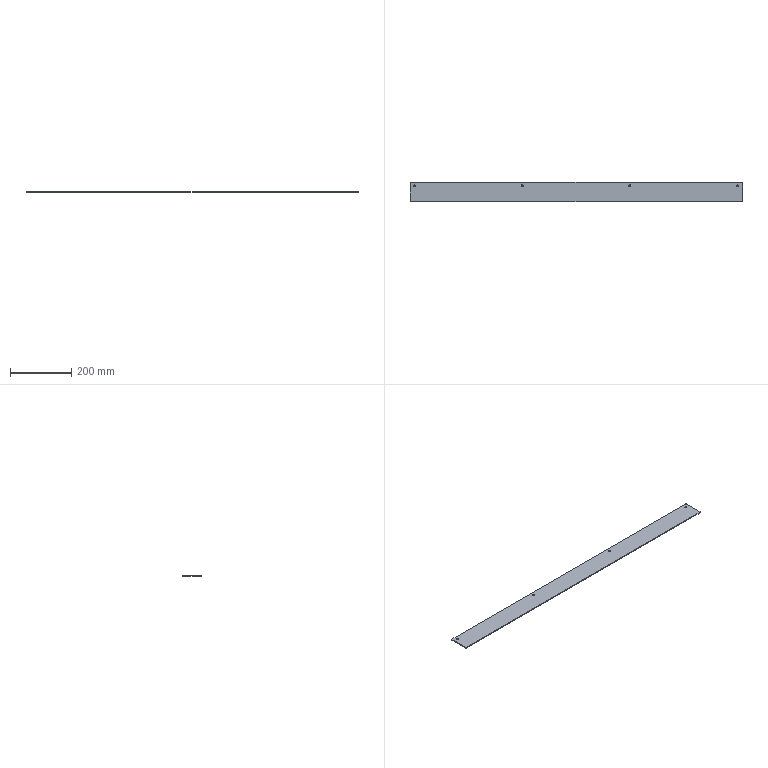Part | NX | features BREP 1 | 1 solid | 18 faces | box 1080 x 65 x 3 mm | volume 210250 mm3 | cylinder 12 | plane 6 | commonest cylinder face diameters 6 x8 4 x4
STEP:
#1=CARTESIAN_POINT('',(540.,-30.5,-3.));
#2=VERTEX_POINT('',#1);
#3=CARTESIAN_POINT('',(538.,-32.5,-3.));
#4=VERTEX_POINT('',#3);
#5=CARTESIAN_POINT('',(538.,-30.5,-3.));
#6=DIRECTION('',(0.,0.,-1.));
#7=DIRECTION('',(-1.,0.,0.));
#8=AXIS2_PLACEMENT_3D('',#5,#6,#7);
#9=CIRCLE('',#8,2.);
#10=EDGE_CURVE('',#2,#4,#9,.T.);
#11=ORIENTED_EDGE('',*,*,#10,.F.);
#12=CARTESIAN_POINT('',(540.,-30.5,0.));
#13=VERTEX_POINT('',#12);
#14=CARTESIAN_POINT('',(540.,-30.5,-3.));
#15=DIRECTION('',(0.,0.,-1.));
#16=VECTOR('',#15,1000.);
#17=LINE('',#14,#16);
#18=EDGE_CURVE('',#13,#2,#17,.T.);
#19=ORIENTED_EDGE('',*,*,#18,.F.);
#20=CARTESIAN_POINT('',(538.,-32.5,0.));
#21=VERTEX_POINT('',#20);
#22=CARTESIAN_POINT('',(538.,-30.5,0.));
#23=DIRECTION('',(0.,0.,1.));
#24=DIRECTION('',(-1.,0.,0.));
#25=AXIS2_PLACEMENT_3D('',#22,#23,#24);
#26=CIRCLE('',#25,2.);
#27=EDGE_CURVE('',#21,#13,#26,.T.);
#28=ORIENTED_EDGE('',*,*,#27,.F.);
#29=CARTESIAN_POINT('',(538.,-32.5,-3.));
#30=DIRECTION('',(0.,0.,1.));
#31=VECTOR('',#30,1000.);
#32=LINE('',#29,#31);
#33=EDGE_CURVE('',#4,#21,#32,.T.);
#34=ORIENTED_EDGE('',*,*,#33,.F.);
#35=EDGE_LOOP('',(#11,#19,#28,#34));
#36=FACE_BOUND('',#35,.T.);
#37=CARTESIAN_POINT('',(538.,-30.5,-3.));
#38=DIRECTION('',(0.,0.,1.));
#39=DIRECTION('',(1.,0.,0.));
#40=AXIS2_PLACEMENT_3D('',#37,#38,#39);
#41=CYLINDRICAL_SURFACE('',#40,2.);
#42=ADVANCED_FACE('',(#36),#41,.T.);
#43=CARTESIAN_POINT('',(538.,32.5,-3.));
#44=VERTEX_POINT('',#43);
#45=CARTESIAN_POINT('',(540.,30.5,-3.));
#46=VERTEX_POINT('',#45);
#47=CARTESIAN_POINT('',(538.,30.5,-3.));
#48=DIRECTION('',(0.,0.,-1.));
#49=DIRECTION('',(-1.,0.,0.));
#50=AXIS2_PLACEMENT_3D('',#47,#48,#49);
#51=CIRCLE('',#50,2.);
#52=EDGE_CURVE('',#44,#46,#51,.T.);
#53=ORIENTED_EDGE('',*,*,#52,.F.);
#54=CARTESIAN_POINT('',(538.,32.5,0.));
#55=VERTEX_POINT('',#54);
#56=CARTESIAN_POINT('',(538.,32.5,-3.));
#57=DIRECTION('',(0.,0.,-1.));
#58=VECTOR('',#57,1000.);
#59=LINE('',#56,#58);
#60=EDGE_CURVE('',#55,#44,#59,.T.);
#61=ORIENTED_EDGE('',*,*,#60,.F.);
#62=CARTESIAN_POINT('',(540.,30.5,0.));
#63=VERTEX_POINT('',#62);
#64=CARTESIAN_POINT('',(538.,30.5,0.));
#65=DIRECTION('',(0.,0.,1.));
#66=DIRECTION('',(-1.,0.,0.));
#67=AXIS2_PLACEMENT_3D('',#64,#65,#66);
#68=CIRCLE('',#67,2.);
#69=EDGE_CURVE('',#63,#55,#68,.T.);
#70=ORIENTED_EDGE('',*,*,#69,.F.);
#71=CARTESIAN_POINT('',(540.,30.5,-3.));
#72=DIRECTION('',(0.,0.,1.));
#73=VECTOR('',#72,1000.);
#74=LINE('',#71,#73);
#75=EDGE_CURVE('',#46,#63,#74,.T.);
#76=ORIENTED_EDGE('',*,*,#75,.F.);
#77=EDGE_LOOP('',(#53,#61,#70,#76));
#78=FACE_BOUND('',#77,.T.);
#79=CARTESIAN_POINT('',(538.,30.5,-3.));
#80=DIRECTION('',(0.,0.,1.));
#81=DIRECTION('',(1.,0.,0.));
#82=AXIS2_PLACEMENT_3D('',#79,#80,#81);
#83=CYLINDRICAL_SURFACE('',#82,2.);
#84=ADVANCED_FACE('',(#78),#83,.T.);
#85=CARTESIAN_POINT('',(-538.,-32.5,-3.));
#86=VERTEX_POINT('',#85);
#87=CARTESIAN_POINT('',(-540.,-30.5,-3.));
#88=VERTEX_POINT('',#87);
#89=CARTESIAN_POINT('',(-538.,-30.5,-3.));
#90=DIRECTION('',(0.,0.,-1.));
#91=DIRECTION('',(-1.,0.,0.));
#92=AXIS2_PLACEMENT_3D('',#89,#90,#91);
#93=CIRCLE('',#92,2.);
#94=EDGE_CURVE('',#86,#88,#93,.T.);
#95=ORIENTED_EDGE('',*,*,#94,.F.);
#96=CARTESIAN_POINT('',(-538.,-32.5,0.));
#97=VERTEX_POINT('',#96);
#98=CARTESIAN_POINT('',(-538.,-32.5,-3.));
#99=DIRECTION('',(0.,0.,-1.));
#100=VECTOR('',#99,1000.);
#101=LINE('',#98,#100);
#102=EDGE_CURVE('',#97,#86,#101,.T.);
#103=ORIENTED_EDGE('',*,*,#102,.F.);
#104=CARTESIAN_POINT('',(-540.,-30.5,0.));
#105=VERTEX_POINT('',#104);
#106=CARTESIAN_POINT('',(-538.,-30.5,0.));
#107=DIRECTION('',(0.,0.,1.));
#108=DIRECTION('',(-1.,0.,0.));
#109=AXIS2_PLACEMENT_3D('',#106,#107,#108);
#110=CIRCLE('',#109,2.);
#111=EDGE_CURVE('',#105,#97,#110,.T.);
#112=ORIENTED_EDGE('',*,*,#111,.F.);
#113=CARTESIAN_POINT('',(-540.,-30.5,-3.));
#114=DIRECTION('',(0.,0.,1.));
#115=VECTOR('',#114,1000.);
#116=LINE('',#113,#115);
#117=EDGE_CURVE('',#88,#105,#116,.T.);
#118=ORIENTED_EDGE('',*,*,#117,.F.);
#119=EDGE_LOOP('',(#95,#103,#112,#118));
#120=FACE_BOUND('',#119,.T.);
#121=CARTESIAN_POINT('',(-538.,-30.5,-3.));
#122=DIRECTION('',(0.,0.,1.));
#123=DIRECTION('',(1.,0.,0.));
#124=AXIS2_PLACEMENT_3D('',#121,#122,#123);
#125=CYLINDRICAL_SURFACE('',#124,2.);
#126=ADVANCED_FACE('',(#120),#125,.T.);
#127=CARTESIAN_POINT('',(-540.,30.5,-3.));
#128=VERTEX_POINT('',#127);
#129=CARTESIAN_POINT('',(-538.,32.5,-3.));
#130=VERTEX_POINT('',#129);
#131=CARTESIAN_POINT('',(-538.,30.5,-3.));
#132=DIRECTION('',(0.,0.,-1.));
#133=DIRECTION('',(-1.,0.,0.));
#134=AXIS2_PLACEMENT_3D('',#131,#132,#133);
#135=CIRCLE('',#134,2.);
#136=EDGE_CURVE('',#128,#130,#135,.T.);
#137=ORIENTED_EDGE('',*,*,#136,.F.);
#138=CARTESIAN_POINT('',(-540.,30.5,0.));
#139=VERTEX_POINT('',#138);
#140=CARTESIAN_POINT('',(-540.,30.5,-3.));
#141=DIRECTION('',(0.,0.,-1.));
#142=VECTOR('',#141,1000.);
#143=LINE('',#140,#142);
#144=EDGE_CURVE('',#139,#128,#143,.T.);
#145=ORIENTED_EDGE('',*,*,#144,.F.);
#146=CARTESIAN_POINT('',(-538.,32.5,0.));
#147=VERTEX_POINT('',#146);
#148=CARTESIAN_POINT('',(-538.,30.5,0.));
#149=DIRECTION('',(0.,0.,1.));
#150=DIRECTION('',(-1.,0.,0.));
#151=AXIS2_PLACEMENT_3D('',#148,#149,#150);
#152=CIRCLE('',#151,2.);
#153=EDGE_CURVE('',#147,#139,#152,.T.);
#154=ORIENTED_EDGE('',*,*,#153,.F.);
#155=CARTESIAN_POINT('',(-538.,32.5,-3.));
#156=DIRECTION('',(0.,0.,1.));
#157=VECTOR('',#156,1000.);
#158=LINE('',#155,#157);
#159=EDGE_CURVE('',#130,#147,#158,.T.);
#160=ORIENTED_EDGE('',*,*,#159,.F.);
#161=EDGE_LOOP('',(#137,#145,#154,#160));
#162=FACE_BOUND('',#161,.T.);
#163=CARTESIAN_POINT('',(-538.,30.5,-3.));
#164=DIRECTION('',(0.,0.,1.));
#165=DIRECTION('',(1.,0.,0.));
#166=AXIS2_PLACEMENT_3D('',#163,#164,#165);
#167=CYLINDRICAL_SURFACE('',#166,2.);
#168=ADVANCED_FACE('',(#162),#167,.T.);
#169=CARTESIAN_POINT('',(528.,20.,0.));
#170=VERTEX_POINT('',#169);
#171=CARTESIAN_POINT('',(528.,20.,-3.));
#172=VERTEX_POINT('',#171);
#173=CARTESIAN_POINT('',(528.,20.,-3.));
#174=DIRECTION('',(0.,0.,-1.));
#175=VECTOR('',#174,1000.);
#176=LINE('',#173,#175);
#177=EDGE_CURVE('',#170,#172,#176,.T.);
#178=ORIENTED_EDGE('',*,*,#177,.F.);
#179=CARTESIAN_POINT('',(522.,20.,0.));
#180=VERTEX_POINT('',#179);
#181=CARTESIAN_POINT('',(525.,20.,0.));
#182=DIRECTION('',(0.,0.,-1.));
#183=DIRECTION('',(-1.,0.,0.));
#184=AXIS2_PLACEMENT_3D('',#181,#182,#183);
#185=CIRCLE('',#184,3.);
#186=EDGE_CURVE('',#180,#170,#185,.T.);
#187=ORIENTED_EDGE('',*,*,#186,.F.);
#188=CARTESIAN_POINT('',(522.,20.,-3.));
#189=VERTEX_POINT('',#188);
#190=CARTESIAN_POINT('',(522.,20.,-3.));
#191=DIRECTION('',(0.,0.,-1.));
#192=VECTOR('',#191,1000.);
#193=LINE('',#190,#192);
#194=EDGE_CURVE('',#180,#189,#193,.T.);
#195=ORIENTED_EDGE('',*,*,#194,.T.);
#196=CARTESIAN_POINT('',(525.,20.,-3.));
#197=DIRECTION('',(0.,0.,-1.));
#198=DIRECTION('',(-1.,0.,0.));
#199=AXIS2_PLACEMENT_3D('',#196,#197,#198);
#200=CIRCLE('',#199,3.);
#201=EDGE_CURVE('',#189,#172,#200,.T.);
#202=ORIENTED_EDGE('',*,*,#201,.T.);
#203=EDGE_LOOP('',(#178,#187,#195,#202));
#204=FACE_BOUND('',#203,.T.);
#205=CARTESIAN_POINT('',(525.,20.,-3.));
#206=DIRECTION('',(0.,0.,-1.));
#207=DIRECTION('',(-1.,0.,0.));
#208=AXIS2_PLACEMENT_3D('',#205,#206,#207);
#209=CYLINDRICAL_SURFACE('',#208,3.);
#210=ADVANCED_FACE('',(#204),#209,.F.);
#211=CARTESIAN_POINT('',(178.,20.,0.));
#212=VERTEX_POINT('',#211);
#213=CARTESIAN_POINT('',(178.,20.,-3.));
#214=VERTEX_POINT('',#213);
#215=CARTESIAN_POINT('',(178.,20.,-3.));
#216=DIRECTION('',(0.,0.,-1.));
#217=VECTOR('',#216,1000.);
#218=LINE('',#215,#217);
#219=EDGE_CURVE('',#212,#214,#218,.T.);
#220=ORIENTED_EDGE('',*,*,#219,.F.);
#221=CARTESIAN_POINT('',(172.,20.,0.));
#222=VERTEX_POINT('',#221);
#223=CARTESIAN_POINT('',(175.,20.,0.));
#224=DIRECTION('',(0.,0.,-1.));
#225=DIRECTION('',(-1.,0.,0.));
#226=AXIS2_PLACEMENT_3D('',#223,#224,#225);
#227=CIRCLE('',#226,3.);
#228=EDGE_CURVE('',#222,#212,#227,.T.);
#229=ORIENTED_EDGE('',*,*,#228,.F.);
#230=CARTESIAN_POINT('',(172.,20.,-3.));
#231=VERTEX_POINT('',#230);
#232=CARTESIAN_POINT('',(172.,20.,-3.));
#233=DIRECTION('',(0.,0.,-1.));
#234=VECTOR('',#233,1000.);
#235=LINE('',#232,#234);
#236=EDGE_CURVE('',#222,#231,#235,.T.);
#237=ORIENTED_EDGE('',*,*,#236,.T.);
#238=CARTESIAN_POINT('',(175.,20.,-3.));
#239=DIRECTION('',(0.,0.,-1.));
#240=DIRECTION('',(-1.,0.,0.));
#241=AXIS2_PLACEMENT_3D('',#238,#239,#240);
#242=CIRCLE('',#241,3.);
#243=EDGE_CURVE('',#231,#214,#242,.T.);
#244=ORIENTED_EDGE('',*,*,#243,.T.);
#245=EDGE_LOOP('',(#220,#229,#237,#244));
#246=FACE_BOUND('',#245,.T.);
#247=CARTESIAN_POINT('',(175.,20.,-3.));
#248=DIRECTION('',(0.,0.,-1.));
#249=DIRECTION('',(-1.,0.,0.));
#250=AXIS2_PLACEMENT_3D('',#247,#248,#249);
#251=CYLINDRICAL_SURFACE('',#250,3.);
#252=ADVANCED_FACE('',(#246),#251,.F.);
#253=CARTESIAN_POINT('',(-172.,20.,0.));
#254=VERTEX_POINT('',#253);
#255=CARTESIAN_POINT('',(-172.,20.,-3.));
#256=VERTEX_POINT('',#255);
#257=CARTESIAN_POINT('',(-172.,20.,-3.));
#258=DIRECTION('',(0.,0.,-1.));
#259=VECTOR('',#258,1000.);
#260=LINE('',#257,#259);
#261=EDGE_CURVE('',#254,#256,#260,.T.);
#262=ORIENTED_EDGE('',*,*,#261,.F.);
#263=CARTESIAN_POINT('',(-178.,20.,0.));
#264=VERTEX_POINT('',#263);
#265=CARTESIAN_POINT('',(-175.,20.,0.));
#266=DIRECTION('',(0.,0.,-1.));
#267=DIRECTION('',(-1.,0.,0.));
#268=AXIS2_PLACEMENT_3D('',#265,#266,#267);
#269=CIRCLE('',#268,3.);
#270=EDGE_CURVE('',#264,#254,#269,.T.);
#271=ORIENTED_EDGE('',*,*,#270,.F.);
#272=CARTESIAN_POINT('',(-178.,20.,-3.));
#273=VERTEX_POINT('',#272);
#274=CARTESIAN_POINT('',(-178.,20.,-3.));
#275=DIRECTION('',(0.,0.,-1.));
#276=VECTOR('',#275,1000.);
#277=LINE('',#274,#276);
#278=EDGE_CURVE('',#264,#273,#277,.T.);
#279=ORIENTED_EDGE('',*,*,#278,.T.);
#280=CARTESIAN_POINT('',(-175.,20.,-3.));
#281=DIRECTION('',(0.,0.,-1.));
#282=DIRECTION('',(-1.,0.,0.));
#283=AXIS2_PLACEMENT_3D('',#280,#281,#282);
#284=CIRCLE('',#283,3.);
#285=EDGE_CURVE('',#273,#256,#284,.T.);
#286=ORIENTED_EDGE('',*,*,#285,.T.);
#287=EDGE_LOOP('',(#262,#271,#279,#286));
#288=FACE_BOUND('',#287,.T.);
#289=CARTESIAN_POINT('',(-175.,20.,-3.));
#290=DIRECTION('',(0.,0.,-1.));
#291=DIRECTION('',(-1.,0.,0.));
#292=AXIS2_PLACEMENT_3D('',#289,#290,#291);
#293=CYLINDRICAL_SURFACE('',#292,3.);
#294=ADVANCED_FACE('',(#288),#293,.F.);
#295=CARTESIAN_POINT('',(-522.,20.,0.));
#296=VERTEX_POINT('',#295);
#297=CARTESIAN_POINT('',(-522.,20.,-3.));
#298=VERTEX_POINT('',#297);
#299=CARTESIAN_POINT('',(-522.,20.,-3.));
#300=DIRECTION('',(0.,0.,-1.));
#301=VECTOR('',#300,1000.);
#302=LINE('',#299,#301);
#303=EDGE_CURVE('',#296,#298,#302,.T.);
#304=ORIENTED_EDGE('',*,*,#303,.F.);
#305=CARTESIAN_POINT('',(-528.,20.,0.));
#306=VERTEX_POINT('',#305);
#307=CARTESIAN_POINT('',(-525.,20.,0.));
#308=DIRECTION('',(0.,0.,-1.));
#309=DIRECTION('',(-1.,0.,0.));
#310=AXIS2_PLACEMENT_3D('',#307,#308,#309);
#311=CIRCLE('',#310,3.);
#312=EDGE_CURVE('',#306,#296,#311,.T.);
#313=ORIENTED_EDGE('',*,*,#312,.F.);
#314=CARTESIAN_POINT('',(-528.,20.,-3.));
#315=VERTEX_POINT('',#314);
#316=CARTESIAN_POINT('',(-528.,20.,-3.));
#317=DIRECTION('',(0.,0.,-1.));
#318=VECTOR('',#317,1000.);
#319=LINE('',#316,#318);
#320=EDGE_CURVE('',#306,#315,#319,.T.);
#321=ORIENTED_EDGE('',*,*,#320,.T.);
#322=CARTESIAN_POINT('',(-525.,20.,-3.));
#323=DIRECTION('',(0.,0.,-1.));
#324=DIRECTION('',(-1.,0.,0.));
#325=AXIS2_PLACEMENT_3D('',#322,#323,#324);
#326=CIRCLE('',#325,3.);
#327=EDGE_CURVE('',#315,#298,#326,.T.);
#328=ORIENTED_EDGE('',*,*,#327,.T.);
#329=EDGE_LOOP('',(#304,#313,#321,#328));
#330=FACE_BOUND('',#329,.T.);
#331=CARTESIAN_POINT('',(-525.,20.,-3.));
#332=DIRECTION('',(0.,0.,-1.));
#333=DIRECTION('',(-1.,0.,0.));
#334=AXIS2_PLACEMENT_3D('',#331,#332,#333);
#335=CYLINDRICAL_SURFACE('',#334,3.);
#336=ADVANCED_FACE('',(#330),#335,.F.);
#337=CARTESIAN_POINT('',(-540.,32.5,0.));
#338=DIRECTION('',(-1.,0.,0.));
#339=VECTOR('',#338,1000.);
#340=LINE('',#337,#339);
#341=EDGE_CURVE('',#55,#147,#340,.T.);
#342=ORIENTED_EDGE('',*,*,#341,.T.);
#343=ORIENTED_EDGE('',*,*,#153,.T.);
#344=CARTESIAN_POINT('',(-540.,-32.5,0.));
#345=DIRECTION('',(0.,-1.,0.));
#346=VECTOR('',#345,1000.);
#347=LINE('',#344,#346);
#348=EDGE_CURVE('',#139,#105,#347,.T.);
#349=ORIENTED_EDGE('',*,*,#348,.T.);
#350=ORIENTED_EDGE('',*,*,#111,.T.);
#351=CARTESIAN_POINT('',(-540.,-32.5,0.));
#352=DIRECTION('',(1.,0.,0.));
#353=VECTOR('',#352,1000.);
#354=LINE('',#351,#353);
#355=EDGE_CURVE('',#97,#21,#354,.T.);
#356=ORIENTED_EDGE('',*,*,#355,.T.);
#357=ORIENTED_EDGE('',*,*,#27,.T.);
#358=CARTESIAN_POINT('',(540.,-32.5,0.));
#359=DIRECTION('',(0.,1.,0.));
#360=VECTOR('',#359,1000.);
#361=LINE('',#358,#360);
#362=EDGE_CURVE('',#13,#63,#361,.T.);
#363=ORIENTED_EDGE('',*,*,#362,.T.);
#364=ORIENTED_EDGE('',*,*,#69,.T.);
#365=EDGE_LOOP('',(#342,#343,#349,#350,#356,#357,#363,#364));
#366=FACE_BOUND('',#365,.T.);
#367=ORIENTED_EDGE('',*,*,#312,.T.);
#368=CARTESIAN_POINT('',(-525.,20.,0.));
#369=DIRECTION('',(0.,0.,-1.));
#370=DIRECTION('',(-1.,0.,0.));
#371=AXIS2_PLACEMENT_3D('',#368,#369,#370);
#372=CIRCLE('',#371,3.);
#373=EDGE_CURVE('',#296,#306,#372,.T.);
#374=ORIENTED_EDGE('',*,*,#373,.T.);
#375=EDGE_LOOP('',(#367,#374));
#376=FACE_BOUND('',#375,.T.);
#377=ORIENTED_EDGE('',*,*,#270,.T.);
#378=CARTESIAN_POINT('',(-175.,20.,0.));
#379=DIRECTION('',(0.,0.,-1.));
#380=DIRECTION('',(-1.,0.,0.));
#381=AXIS2_PLACEMENT_3D('',#378,#379,#380);
#382=CIRCLE('',#381,3.);
#383=EDGE_CURVE('',#254,#264,#382,.T.);
#384=ORIENTED_EDGE('',*,*,#383,.T.);
#385=EDGE_LOOP('',(#377,#384));
#386=FACE_BOUND('',#385,.T.);
#387=ORIENTED_EDGE('',*,*,#228,.T.);
#388=CARTESIAN_POINT('',(175.,20.,0.));
#389=DIRECTION('',(0.,0.,-1.));
#390=DIRECTION('',(-1.,0.,0.));
#391=AXIS2_PLACEMENT_3D('',#388,#389,#390);
#392=CIRCLE('',#391,3.);
#393=EDGE_CURVE('',#212,#222,#392,.T.);
#394=ORIENTED_EDGE('',*,*,#393,.T.);
#395=EDGE_LOOP('',(#387,#394));
#396=FACE_BOUND('',#395,.T.);
#397=ORIENTED_EDGE('',*,*,#186,.T.);
#398=CARTESIAN_POINT('',(525.,20.,0.));
#399=DIRECTION('',(0.,0.,-1.));
#400=DIRECTION('',(-1.,0.,0.));
#401=AXIS2_PLACEMENT_3D('',#398,#399,#400);
#402=CIRCLE('',#401,3.);
#403=EDGE_CURVE('',#170,#180,#402,.T.);
#404=ORIENTED_EDGE('',*,*,#403,.T.);
#405=EDGE_LOOP('',(#397,#404));
#406=FACE_BOUND('',#405,.T.);
#407=CARTESIAN_POINT('',(0.,0.,0.));
#408=DIRECTION('',(0.,0.,-1.));
#409=DIRECTION('',(-1.,0.,0.));
#410=AXIS2_PLACEMENT_3D('',#407,#408,#409);
#411=PLANE('',#410);
#412=ADVANCED_FACE('',(#366,#376,#386,#396,#406),#411,.F.);
#413=CARTESIAN_POINT('',(-540.,-32.5,-3.));
#414=DIRECTION('',(0.,-1.,0.));
#415=VECTOR('',#414,1000.);
#416=LINE('',#413,#415);
#417=EDGE_CURVE('',#128,#88,#416,.T.);
#418=ORIENTED_EDGE('',*,*,#417,.F.);
#419=ORIENTED_EDGE('',*,*,#136,.T.);
#420=CARTESIAN_POINT('',(-540.,32.5,-3.));
#421=DIRECTION('',(-1.,0.,0.));
#422=VECTOR('',#421,1000.);
#423=LINE('',#420,#422);
#424=EDGE_CURVE('',#44,#130,#423,.T.);
#425=ORIENTED_EDGE('',*,*,#424,.F.);
#426=ORIENTED_EDGE('',*,*,#52,.T.);
#427=CARTESIAN_POINT('',(540.,-32.5,-3.));
#428=DIRECTION('',(0.,1.,0.));
#429=VECTOR('',#428,1000.);
#430=LINE('',#427,#429);
#431=EDGE_CURVE('',#2,#46,#430,.T.);
#432=ORIENTED_EDGE('',*,*,#431,.F.);
#433=ORIENTED_EDGE('',*,*,#10,.T.);
#434=CARTESIAN_POINT('',(-540.,-32.5,-3.));
#435=DIRECTION('',(1.,0.,0.));
#436=VECTOR('',#435,1000.);
#437=LINE('',#434,#436);
#438=EDGE_CURVE('',#86,#4,#437,.T.);
#439=ORIENTED_EDGE('',*,*,#438,.F.);
#440=ORIENTED_EDGE('',*,*,#94,.T.);
#441=EDGE_LOOP('',(#418,#419,#425,#426,#432,#433,#439,#440));
#442=FACE_BOUND('',#441,.T.);
#443=ORIENTED_EDGE('',*,*,#327,.F.);
#444=CARTESIAN_POINT('',(-525.,20.,-3.));
#445=DIRECTION('',(0.,0.,-1.));
#446=DIRECTION('',(-1.,0.,0.));
#447=AXIS2_PLACEMENT_3D('',#444,#445,#446);
#448=CIRCLE('',#447,3.);
#449=EDGE_CURVE('',#298,#315,#448,.T.);
#450=ORIENTED_EDGE('',*,*,#449,.F.);
#451=EDGE_LOOP('',(#443,#450));
#452=FACE_BOUND('',#451,.T.);
#453=ORIENTED_EDGE('',*,*,#285,.F.);
#454=CARTESIAN_POINT('',(-175.,20.,-3.));
#455=DIRECTION('',(0.,0.,-1.));
#456=DIRECTION('',(-1.,0.,0.));
#457=AXIS2_PLACEMENT_3D('',#454,#455,#456);
#458=CIRCLE('',#457,3.);
#459=EDGE_CURVE('',#256,#273,#458,.T.);
#460=ORIENTED_EDGE('',*,*,#459,.F.);
#461=EDGE_LOOP('',(#453,#460));
#462=FACE_BOUND('',#461,.T.);
#463=ORIENTED_EDGE('',*,*,#243,.F.);
#464=CARTESIAN_POINT('',(175.,20.,-3.));
#465=DIRECTION('',(0.,0.,-1.));
#466=DIRECTION('',(-1.,0.,0.));
#467=AXIS2_PLACEMENT_3D('',#464,#465,#466);
#468=CIRCLE('',#467,3.);
#469=EDGE_CURVE('',#214,#231,#468,.T.);
#470=ORIENTED_EDGE('',*,*,#469,.F.);
#471=EDGE_LOOP('',(#463,#470));
#472=FACE_BOUND('',#471,.T.);
#473=ORIENTED_EDGE('',*,*,#201,.F.);
#474=CARTESIAN_POINT('',(525.,20.,-3.));
#475=DIRECTION('',(0.,0.,-1.));
#476=DIRECTION('',(-1.,0.,0.));
#477=AXIS2_PLACEMENT_3D('',#474,#475,#476);
#478=CIRCLE('',#477,3.);
#479=EDGE_CURVE('',#172,#189,#478,.T.);
#480=ORIENTED_EDGE('',*,*,#479,.F.);
#481=EDGE_LOOP('',(#473,#480));
#482=FACE_BOUND('',#481,.T.);
#483=CARTESIAN_POINT('',(0.,0.,-3.));
#484=DIRECTION('',(0.,0.,-1.));
#485=DIRECTION('',(-1.,0.,0.));
#486=AXIS2_PLACEMENT_3D('',#483,#484,#485);
#487=PLANE('',#486);
#488=ADVANCED_FACE('',(#442,#452,#462,#472,#482),#487,.T.);
#489=ORIENTED_EDGE('',*,*,#424,.T.);
#490=ORIENTED_EDGE('',*,*,#159,.T.);
#491=ORIENTED_EDGE('',*,*,#341,.F.);
#492=ORIENTED_EDGE('',*,*,#60,.T.);
#493=EDGE_LOOP('',(#489,#490,#491,#492));
#494=FACE_BOUND('',#493,.T.);
#495=CARTESIAN_POINT('',(-540.,32.5,-3.));
#496=DIRECTION('',(0.,1.,0.));
#497=DIRECTION('',(0.,0.,1.));
#498=AXIS2_PLACEMENT_3D('',#495,#496,#497);
#499=PLANE('',#498);
#500=ADVANCED_FACE('',(#494),#499,.T.);
#501=ORIENTED_EDGE('',*,*,#348,.F.);
#502=ORIENTED_EDGE('',*,*,#144,.T.);
#503=ORIENTED_EDGE('',*,*,#417,.T.);
#504=ORIENTED_EDGE('',*,*,#117,.T.);
#505=EDGE_LOOP('',(#501,#502,#503,#504));
#506=FACE_BOUND('',#505,.T.);
#507=CARTESIAN_POINT('',(-540.,-32.5,-3.));
#508=DIRECTION('',(-1.,0.,0.));
#509=DIRECTION('',(0.,0.,1.));
#510=AXIS2_PLACEMENT_3D('',#507,#508,#509);
#511=PLANE('',#510);
#512=ADVANCED_FACE('',(#506),#511,.T.);
#513=ORIENTED_EDGE('',*,*,#355,.F.);
#514=ORIENTED_EDGE('',*,*,#102,.T.);
#515=ORIENTED_EDGE('',*,*,#438,.T.);
#516=ORIENTED_EDGE('',*,*,#33,.T.);
#517=EDGE_LOOP('',(#513,#514,#515,#516));
#518=FACE_BOUND('',#517,.T.);
#519=CARTESIAN_POINT('',(-540.,-32.5,-3.));
#520=DIRECTION('',(0.,-1.,0.));
#521=DIRECTION('',(0.,0.,-1.));
#522=AXIS2_PLACEMENT_3D('',#519,#520,#521);
#523=PLANE('',#522);
#524=ADVANCED_FACE('',(#518),#523,.T.);
#525=ORIENTED_EDGE('',*,*,#431,.T.);
#526=ORIENTED_EDGE('',*,*,#75,.T.);
#527=ORIENTED_EDGE('',*,*,#362,.F.);
#528=ORIENTED_EDGE('',*,*,#18,.T.);
#529=EDGE_LOOP('',(#525,#526,#527,#528));
#530=FACE_BOUND('',#529,.T.);
#531=CARTESIAN_POINT('',(540.,-32.5,-3.));
#532=DIRECTION('',(1.,0.,0.));
#533=DIRECTION('',(0.,0.,-1.));
#534=AXIS2_PLACEMENT_3D('',#531,#532,#533);
#535=PLANE('',#534);
#536=ADVANCED_FACE('',(#530),#535,.T.);
#537=ORIENTED_EDGE('',*,*,#373,.F.);
#538=ORIENTED_EDGE('',*,*,#303,.T.);
#539=ORIENTED_EDGE('',*,*,#449,.T.);
#540=ORIENTED_EDGE('',*,*,#320,.F.);
#541=EDGE_LOOP('',(#537,#538,#539,#540));
#542=FACE_BOUND('',#541,.T.);
#543=CARTESIAN_POINT('',(-525.,20.,-3.));
#544=DIRECTION('',(0.,0.,-1.));
#545=DIRECTION('',(-1.,0.,0.));
#546=AXIS2_PLACEMENT_3D('',#543,#544,#545);
#547=CYLINDRICAL_SURFACE('',#546,3.);
#548=ADVANCED_FACE('',(#542),#547,.F.);
#549=ORIENTED_EDGE('',*,*,#383,.F.);
#550=ORIENTED_EDGE('',*,*,#261,.T.);
#551=ORIENTED_EDGE('',*,*,#459,.T.);
#552=ORIENTED_EDGE('',*,*,#278,.F.);
#553=EDGE_LOOP('',(#549,#550,#551,#552));
#554=FACE_BOUND('',#553,.T.);
#555=CARTESIAN_POINT('',(-175.,20.,-3.));
#556=DIRECTION('',(0.,0.,-1.));
#557=DIRECTION('',(-1.,0.,0.));
#558=AXIS2_PLACEMENT_3D('',#555,#556,#557);
#559=CYLINDRICAL_SURFACE('',#558,3.);
#560=ADVANCED_FACE('',(#554),#559,.F.);
#561=ORIENTED_EDGE('',*,*,#393,.F.);
#562=ORIENTED_EDGE('',*,*,#219,.T.);
#563=ORIENTED_EDGE('',*,*,#469,.T.);
#564=ORIENTED_EDGE('',*,*,#236,.F.);
#565=EDGE_LOOP('',(#561,#562,#563,#564));
#566=FACE_BOUND('',#565,.T.);
#567=CARTESIAN_POINT('',(175.,20.,-3.));
#568=DIRECTION('',(0.,0.,-1.));
#569=DIRECTION('',(-1.,0.,0.));
#570=AXIS2_PLACEMENT_3D('',#567,#568,#569);
#571=CYLINDRICAL_SURFACE('',#570,3.);
#572=ADVANCED_FACE('',(#566),#571,.F.);
#573=ORIENTED_EDGE('',*,*,#403,.F.);
#574=ORIENTED_EDGE('',*,*,#177,.T.);
#575=ORIENTED_EDGE('',*,*,#479,.T.);
#576=ORIENTED_EDGE('',*,*,#194,.F.);
#577=EDGE_LOOP('',(#573,#574,#575,#576));
#578=FACE_BOUND('',#577,.T.);
#579=CARTESIAN_POINT('',(525.,20.,-3.));
#580=DIRECTION('',(0.,0.,-1.));
#581=DIRECTION('',(-1.,0.,0.));
#582=AXIS2_PLACEMENT_3D('',#579,#580,#581);
#583=CYLINDRICAL_SURFACE('',#582,3.);
#584=ADVANCED_FACE('',(#578),#583,.F.);
#585=CLOSED_SHELL('',(#42,#84,#126,#168,#210,#252,#294,#336,#412,#488,#500,#512,#524,#536,#548,#560,#572,#584));
#586=MANIFOLD_SOLID_BREP('',#585);
#587=(LENGTH_UNIT()NAMED_UNIT(*)SI_UNIT(.MILLI.,.METRE.));
#588=UNCERTAINTY_MEASURE_WITH_UNIT(LENGTH_MEASURE(0.00001),#587,'','');
#589=(NAMED_UNIT(*)PLANE_ANGLE_UNIT()SI_UNIT($,.RADIAN.));
#590=(NAMED_UNIT(*)SI_UNIT($,.STERADIAN.)SOLID_ANGLE_UNIT());
#591=(GEOMETRIC_REPRESENTATION_CONTEXT(3)GLOBAL_UNCERTAINTY_ASSIGNED_CONTEXT((#588))GLOBAL_UNIT_ASSIGNED_CONTEXT((#587,#589,#590))REPRESENTATION_CONTEXT('',''));
#592=ADVANCED_BREP_SHAPE_REPRESENTATION('',(#586),#591);